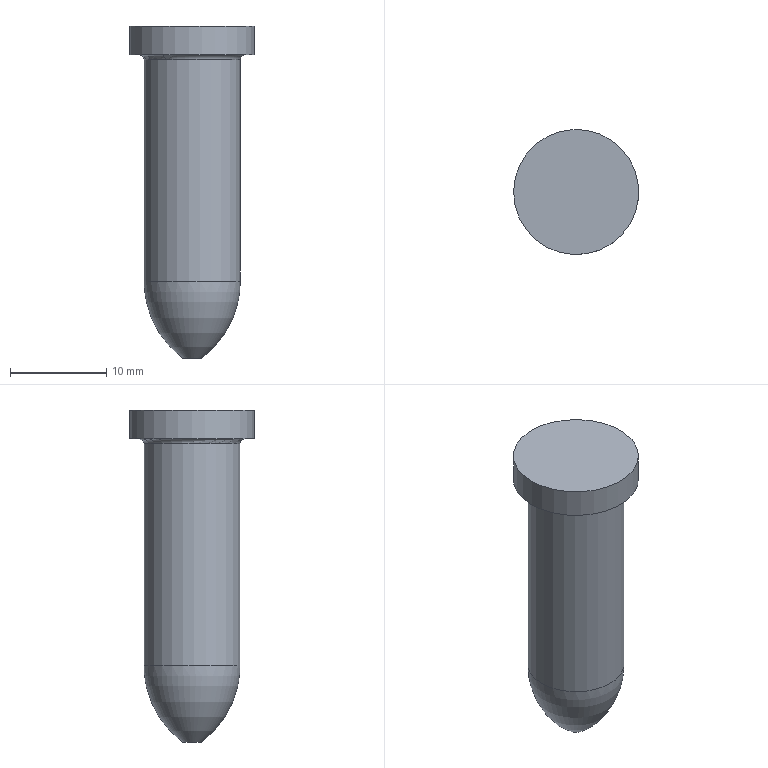Part | NX | features SPT10-26.5-P10.00_1 2 | 1 solid | 7 faces | box 13 x 13 x 34.5 mm | volume 2640 mm3 | plane 3 | cylinder 2 | torus 2 | commonest cylinder face diameters 10 x1 13 x1
STEP:
#1=CARTESIAN_POINT('',(45.468,2.113,-1.5));
#2=VERTEX_POINT('',#1);
#3=CARTESIAN_POINT('',(50.,0.,-1.5));
#4=DIRECTION('',(0.,0.,-1.));
#5=DIRECTION('',(-0.9063,0.4226,0.));
#6=AXIS2_PLACEMENT_3D('',#3,#4,#5);
#7=CIRCLE('',#6,5.);
#8=EDGE_CURVE('',#2,#2,#7,.T.);
#9=ORIENTED_EDGE('',*,*,#8,.F.);
#10=EDGE_LOOP('',(#9));
#11=FACE_BOUND('',#10,.T.);
#12=CARTESIAN_POINT('',(45.468,2.113,21.5));
#13=VERTEX_POINT('',#12);
#14=CARTESIAN_POINT('',(50.,0.,21.5));
#15=DIRECTION('',(0.,0.,1.));
#16=DIRECTION('',(0.9063,-0.4226,0.));
#17=AXIS2_PLACEMENT_3D('',#14,#15,#16);
#18=CIRCLE('',#17,5.);
#19=EDGE_CURVE('',#13,#13,#18,.T.);
#20=ORIENTED_EDGE('',*,*,#19,.F.);
#21=EDGE_LOOP('',(#20));
#22=FACE_BOUND('',#21,.T.);
#23=CARTESIAN_POINT('',(50.,0.,10.25));
#24=DIRECTION('',(0.,0.,-1.));
#25=DIRECTION('',(0.9063,-0.4226,0.));
#26=AXIS2_PLACEMENT_3D('',#23,#24,#25);
#27=CYLINDRICAL_SURFACE('',#26,5.);
#28=ADVANCED_FACE('',(#11,#22),#27,.T.);
#29=ORIENTED_EDGE('',*,*,#19,.T.);
#30=EDGE_LOOP('',(#29));
#31=FACE_BOUND('',#30,.T.);
#32=CARTESIAN_POINT('',(45.015,2.324,22.));
#33=VERTEX_POINT('',#32);
#34=CARTESIAN_POINT('',(50.,0.,22.));
#35=DIRECTION('',(0.,0.,-1.));
#36=DIRECTION('',(0.9063,-0.4226,0.));
#37=AXIS2_PLACEMENT_3D('',#34,#35,#36);
#38=CIRCLE('',#37,5.5);
#39=EDGE_CURVE('',#33,#33,#38,.T.);
#40=ORIENTED_EDGE('',*,*,#39,.T.);
#41=EDGE_LOOP('',(#40));
#42=FACE_BOUND('',#41,.T.);
#43=CARTESIAN_POINT('',(50.,0.,21.5));
#44=DIRECTION('',(0.,0.,1.));
#45=DIRECTION('',(-0.9063,0.4226,0.));
#46=AXIS2_PLACEMENT_3D('',#43,#44,#45);
#47=TOROIDAL_SURFACE('',#46,5.5,0.5);
#48=ADVANCED_FACE('',(#31,#42),#47,.F.);
#49=CARTESIAN_POINT('',(44.109,2.747,22.));
#50=VERTEX_POINT('',#49);
#51=CARTESIAN_POINT('',(50.,0.,22.));
#52=DIRECTION('',(0.,0.,-1.));
#53=DIRECTION('',(-0.9063,0.4226,0.));
#54=AXIS2_PLACEMENT_3D('',#51,#52,#53);
#55=CIRCLE('',#54,6.5);
#56=EDGE_CURVE('',#50,#50,#55,.T.);
#57=ORIENTED_EDGE('',*,*,#56,.T.);
#58=EDGE_LOOP('',(#57));
#59=FACE_BOUND('',#58,.T.);
#60=ORIENTED_EDGE('',*,*,#39,.F.);
#61=EDGE_LOOP('',(#60));
#62=FACE_BOUND('',#61,.T.);
#63=CARTESIAN_POINT('',(50.,0.,22.));
#64=DIRECTION('',(0.,0.,-1.));
#65=DIRECTION('',(0.9063,-0.4226,0.));
#66=AXIS2_PLACEMENT_3D('',#63,#64,#65);
#67=PLANE('',#66);
#68=ADVANCED_FACE('',(#59,#62),#67,.T.);
#69=CARTESIAN_POINT('',(49.094,0.4226,-9.5));
#70=VERTEX_POINT('',#69);
#71=CARTESIAN_POINT('',(50.,0.,-9.5));
#72=DIRECTION('',(0.,0.,1.));
#73=DIRECTION('',(0.9063,-0.4226,0.));
#74=AXIS2_PLACEMENT_3D('',#71,#72,#73);
#75=CIRCLE('',#74,1.);
#76=EDGE_CURVE('',#70,#70,#75,.T.);
#77=ORIENTED_EDGE('',*,*,#76,.F.);
#78=EDGE_LOOP('',(#77));
#79=FACE_BOUND('',#78,.T.);
#80=CARTESIAN_POINT('',(50.,0.,-9.5));
#81=DIRECTION('',(0.,0.,1.));
#82=DIRECTION('',(-0.9063,0.4226,0.));
#83=AXIS2_PLACEMENT_3D('',#80,#81,#82);
#84=PLANE('',#83);
#85=ADVANCED_FACE('',(#79),#84,.F.);
#86=ORIENTED_EDGE('',*,*,#76,.T.);
#87=EDGE_LOOP('',(#86));
#88=FACE_BOUND('',#87,.T.);
#89=ORIENTED_EDGE('',*,*,#8,.T.);
#90=EDGE_LOOP('',(#89));
#91=FACE_BOUND('',#90,.T.);
#92=CARTESIAN_POINT('',(50.,0.,-1.5));
#93=DIRECTION('',(0.,0.,-1.));
#94=DIRECTION('',(0.9063,-0.4226,0.));
#95=AXIS2_PLACEMENT_3D('',#92,#93,#94);
#96=DEGENERATE_TOROIDAL_SURFACE('',#95,5.,10.,.F.);
#97=ADVANCED_FACE('',(#88,#91),#96,.F.);
#98=CARTESIAN_POINT('',(44.109,2.747,25.));
#99=VERTEX_POINT('',#98);
#100=CARTESIAN_POINT('',(50.,0.,25.));
#101=DIRECTION('',(0.,0.,1.));
#102=DIRECTION('',(-0.9063,0.4226,0.));
#103=AXIS2_PLACEMENT_3D('',#100,#101,#102);
#104=CIRCLE('',#103,6.5);
#105=EDGE_CURVE('',#99,#99,#104,.T.);
#106=ORIENTED_EDGE('',*,*,#105,.F.);
#107=EDGE_LOOP('',(#106));
#108=FACE_BOUND('',#107,.T.);
#109=ORIENTED_EDGE('',*,*,#56,.F.);
#110=EDGE_LOOP('',(#109));
#111=FACE_BOUND('',#110,.T.);
#112=CARTESIAN_POINT('',(50.,0.,23.5));
#113=DIRECTION('',(0.,0.,-1.));
#114=DIRECTION('',(0.9063,-0.4226,0.));
#115=AXIS2_PLACEMENT_3D('',#112,#113,#114);
#116=CYLINDRICAL_SURFACE('',#115,6.5);
#117=ADVANCED_FACE('',(#108,#111),#116,.T.);
#118=ORIENTED_EDGE('',*,*,#105,.T.);
#119=EDGE_LOOP('',(#118));
#120=FACE_BOUND('',#119,.T.);
#121=CARTESIAN_POINT('',(50.,0.,25.));
#122=DIRECTION('',(0.,0.,1.));
#123=DIRECTION('',(-0.9063,0.4226,0.));
#124=AXIS2_PLACEMENT_3D('',#121,#122,#123);
#125=PLANE('',#124);
#126=ADVANCED_FACE('',(#120),#125,.T.);
#127=CLOSED_SHELL('',(#28,#48,#68,#85,#97,#117,#126));
#128=MANIFOLD_SOLID_BREP('',#127);
#129=(LENGTH_UNIT()NAMED_UNIT(*)SI_UNIT(.MILLI.,.METRE.));
#130=UNCERTAINTY_MEASURE_WITH_UNIT(LENGTH_MEASURE(0.00001),#129,'','');
#131=(NAMED_UNIT(*)PLANE_ANGLE_UNIT()SI_UNIT($,.RADIAN.));
#132=(NAMED_UNIT(*)SI_UNIT($,.STERADIAN.)SOLID_ANGLE_UNIT());
#133=(GEOMETRIC_REPRESENTATION_CONTEXT(3)GLOBAL_UNCERTAINTY_ASSIGNED_CONTEXT((#130))GLOBAL_UNIT_ASSIGNED_CONTEXT((#129,#131,#132))REPRESENTATION_CONTEXT('',''));
#134=ADVANCED_BREP_SHAPE_REPRESENTATION('',(#128),#133);